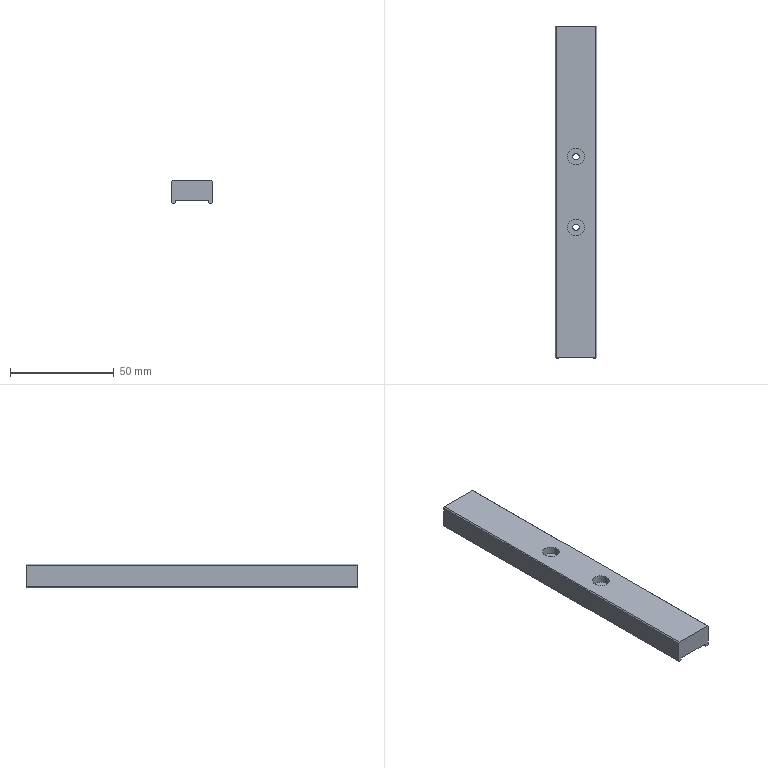Part | NX | features EXTRUDE 3, DATUM_CSYS 1 | 1 solid | 22 faces | box 20.2 x 160 x 11.5 mm | volume 32690 mm3 | plane 18 | cylinder 4 | commonest cylinder face diameters 3 x2 8 x2
STEP:
#1=CARTESIAN_POINT('',(4558.975,6805.349,0.));
#2=VERTEX_POINT('',#1);
#3=CARTESIAN_POINT('',(4578.175,6805.349,0.));
#4=VERTEX_POINT('',#3);
#5=CARTESIAN_POINT('',(4558.975,6805.349,0.));
#6=DIRECTION('',(1.,0.,0.));
#7=VECTOR('',#6,1000.);
#8=LINE('',#5,#7);
#9=EDGE_CURVE('',#2,#4,#8,.T.);
#10=ORIENTED_EDGE('',*,*,#9,.T.);
#11=CARTESIAN_POINT('',(4578.175,6965.349,0.));
#12=VERTEX_POINT('',#11);
#13=CARTESIAN_POINT('',(4578.175,6965.349,0.));
#14=DIRECTION('',(0.,-1.,0.));
#15=VECTOR('',#14,1000.);
#16=LINE('',#13,#15);
#17=EDGE_CURVE('',#12,#4,#16,.T.);
#18=ORIENTED_EDGE('',*,*,#17,.F.);
#19=CARTESIAN_POINT('',(4558.975,6965.349,0.));
#20=VERTEX_POINT('',#19);
#21=CARTESIAN_POINT('',(4558.975,6965.349,0.));
#22=DIRECTION('',(1.,0.,0.));
#23=VECTOR('',#22,1000.);
#24=LINE('',#21,#23);
#25=EDGE_CURVE('',#20,#12,#24,.T.);
#26=ORIENTED_EDGE('',*,*,#25,.F.);
#27=CARTESIAN_POINT('',(4558.975,6965.349,0.));
#28=DIRECTION('',(0.,-1.,0.));
#29=VECTOR('',#28,1000.);
#30=LINE('',#27,#29);
#31=EDGE_CURVE('',#20,#2,#30,.T.);
#32=ORIENTED_EDGE('',*,*,#31,.T.);
#33=EDGE_LOOP('',(#10,#18,#26,#32));
#34=FACE_BOUND('',#33,.T.);
#35=CARTESIAN_POINT('',(4572.575,6902.351,0.));
#36=VERTEX_POINT('',#35);
#37=CARTESIAN_POINT('',(4568.575,6902.351,0.));
#38=DIRECTION('',(0.,0.,-1.));
#39=DIRECTION('',(1.,0.,0.));
#40=AXIS2_PLACEMENT_3D('',#37,#38,#39);
#41=CIRCLE('',#40,4.);
#42=EDGE_CURVE('',#36,#36,#41,.T.);
#43=ORIENTED_EDGE('',*,*,#42,.T.);
#44=EDGE_LOOP('',(#43));
#45=FACE_BOUND('',#44,.T.);
#46=CARTESIAN_POINT('',(4572.575,6868.351,0.));
#47=VERTEX_POINT('',#46);
#48=CARTESIAN_POINT('',(4568.575,6868.351,0.));
#49=DIRECTION('',(0.,0.,1.));
#50=DIRECTION('',(1.,0.,0.));
#51=AXIS2_PLACEMENT_3D('',#48,#49,#50);
#52=CIRCLE('',#51,4.);
#53=EDGE_CURVE('',#47,#47,#52,.T.);
#54=ORIENTED_EDGE('',*,*,#53,.F.);
#55=EDGE_LOOP('',(#54));
#56=FACE_BOUND('',#55,.T.);
#57=CARTESIAN_POINT('',(4558.975,6965.349,0.));
#58=DIRECTION('',(0.,0.,-1.));
#59=DIRECTION('',(-1.,0.,0.));
#60=AXIS2_PLACEMENT_3D('',#57,#58,#59);
#61=PLANE('',#60);
#62=ADVANCED_FACE('',(#34,#45,#56),#61,.F.);
#63=CARTESIAN_POINT('',(4570.075,6868.351,-10.));
#64=VERTEX_POINT('',#63);
#65=CARTESIAN_POINT('',(4568.575,6868.351,-10.));
#66=DIRECTION('',(0.,0.,1.));
#67=DIRECTION('',(1.,0.,0.));
#68=AXIS2_PLACEMENT_3D('',#65,#66,#67);
#69=CIRCLE('',#68,1.5);
#70=EDGE_CURVE('',#64,#64,#69,.F.);
#71=ORIENTED_EDGE('',*,*,#70,.T.);
#72=EDGE_LOOP('',(#71));
#73=FACE_BOUND('',#72,.T.);
#74=CARTESIAN_POINT('',(4570.075,6868.351,-3.8));
#75=VERTEX_POINT('',#74);
#76=CARTESIAN_POINT('',(4568.575,6868.351,-3.8));
#77=DIRECTION('',(0.,0.,1.));
#78=DIRECTION('',(1.,0.,0.));
#79=AXIS2_PLACEMENT_3D('',#76,#77,#78);
#80=CIRCLE('',#79,1.5);
#81=EDGE_CURVE('',#75,#75,#80,.F.);
#82=ORIENTED_EDGE('',*,*,#81,.F.);
#83=EDGE_LOOP('',(#82));
#84=FACE_BOUND('',#83,.T.);
#85=CARTESIAN_POINT('',(4568.575,6868.351,-55000.));
#86=DIRECTION('',(0.,0.,1.));
#87=DIRECTION('',(1.,0.,0.));
#88=AXIS2_PLACEMENT_3D('',#85,#86,#87);
#89=CYLINDRICAL_SURFACE('',#88,1.5);
#90=ADVANCED_FACE('',(#73,#84),#89,.F.);
#91=CARTESIAN_POINT('',(4570.075,6902.351,-10.));
#92=VERTEX_POINT('',#91);
#93=CARTESIAN_POINT('',(4568.575,6902.351,-10.));
#94=DIRECTION('',(0.,0.,1.));
#95=DIRECTION('',(1.,0.,0.));
#96=AXIS2_PLACEMENT_3D('',#93,#94,#95);
#97=CIRCLE('',#96,1.5);
#98=EDGE_CURVE('',#92,#92,#97,.T.);
#99=ORIENTED_EDGE('',*,*,#98,.T.);
#100=EDGE_LOOP('',(#99));
#101=FACE_BOUND('',#100,.T.);
#102=CARTESIAN_POINT('',(4576.675,6805.349,-10.));
#103=VERTEX_POINT('',#102);
#104=CARTESIAN_POINT('',(4560.475,6805.349,-10.));
#105=VERTEX_POINT('',#104);
#106=CARTESIAN_POINT('',(4576.675,6805.349,-10.));
#107=DIRECTION('',(-1.,0.,0.));
#108=VECTOR('',#107,1000.);
#109=LINE('',#106,#108);
#110=EDGE_CURVE('',#103,#105,#109,.T.);
#111=ORIENTED_EDGE('',*,*,#110,.T.);
#112=CARTESIAN_POINT('',(4560.475,6965.349,-10.));
#113=VERTEX_POINT('',#112);
#114=CARTESIAN_POINT('',(4560.475,6965.349,-10.));
#115=DIRECTION('',(0.,-1.,0.));
#116=VECTOR('',#115,1000.);
#117=LINE('',#114,#116);
#118=EDGE_CURVE('',#113,#105,#117,.T.);
#119=ORIENTED_EDGE('',*,*,#118,.F.);
#120=CARTESIAN_POINT('',(4576.675,6965.349,-10.));
#121=VERTEX_POINT('',#120);
#122=CARTESIAN_POINT('',(4576.675,6965.349,-10.));
#123=DIRECTION('',(-1.,0.,0.));
#124=VECTOR('',#123,1000.);
#125=LINE('',#122,#124);
#126=EDGE_CURVE('',#121,#113,#125,.T.);
#127=ORIENTED_EDGE('',*,*,#126,.F.);
#128=CARTESIAN_POINT('',(4576.675,6965.349,-10.));
#129=DIRECTION('',(0.,-1.,0.));
#130=VECTOR('',#129,1000.);
#131=LINE('',#128,#130);
#132=EDGE_CURVE('',#121,#103,#131,.T.);
#133=ORIENTED_EDGE('',*,*,#132,.T.);
#134=EDGE_LOOP('',(#111,#119,#127,#133));
#135=FACE_BOUND('',#134,.T.);
#136=ORIENTED_EDGE('',*,*,#70,.F.);
#137=EDGE_LOOP('',(#136));
#138=FACE_BOUND('',#137,.T.);
#139=CARTESIAN_POINT('',(4576.675,6965.349,-10.));
#140=DIRECTION('',(0.,0.,1.));
#141=DIRECTION('',(1.,0.,0.));
#142=AXIS2_PLACEMENT_3D('',#139,#140,#141);
#143=PLANE('',#142);
#144=ADVANCED_FACE('',(#101,#135,#138),#143,.F.);
#145=CARTESIAN_POINT('',(4578.675,6805.349,-0.5));
#146=VERTEX_POINT('',#145);
#147=CARTESIAN_POINT('',(4578.175,6805.349,0.));
#148=DIRECTION('',(0.7071,0.,-0.7071));
#149=VECTOR('',#148,1000.);
#150=LINE('',#147,#149);
#151=EDGE_CURVE('',#4,#146,#150,.T.);
#152=ORIENTED_EDGE('',*,*,#151,.T.);
#153=CARTESIAN_POINT('',(4578.675,6965.349,-0.5));
#154=VERTEX_POINT('',#153);
#155=CARTESIAN_POINT('',(4578.675,6965.349,-0.5));
#156=DIRECTION('',(0.,-1.,0.));
#157=VECTOR('',#156,1000.);
#158=LINE('',#155,#157);
#159=EDGE_CURVE('',#154,#146,#158,.T.);
#160=ORIENTED_EDGE('',*,*,#159,.F.);
#161=CARTESIAN_POINT('',(4578.175,6965.349,0.));
#162=DIRECTION('',(0.7071,0.,-0.7071));
#163=VECTOR('',#162,1000.);
#164=LINE('',#161,#163);
#165=EDGE_CURVE('',#12,#154,#164,.T.);
#166=ORIENTED_EDGE('',*,*,#165,.F.);
#167=ORIENTED_EDGE('',*,*,#17,.T.);
#168=EDGE_LOOP('',(#152,#160,#166,#167));
#169=FACE_BOUND('',#168,.T.);
#170=CARTESIAN_POINT('',(4578.175,6965.349,0.));
#171=DIRECTION('',(-0.7071,0.,-0.7071));
#172=DIRECTION('',(-0.7071,0.,0.7071));
#173=AXIS2_PLACEMENT_3D('',#170,#171,#172);
#174=PLANE('',#173);
#175=ADVANCED_FACE('',(#169),#174,.F.);
#176=CARTESIAN_POINT('',(4578.675,6805.349,-11.));
#177=VERTEX_POINT('',#176);
#178=CARTESIAN_POINT('',(4578.675,6805.349,-0.5));
#179=DIRECTION('',(0.,0.,-1.));
#180=VECTOR('',#179,1000.);
#181=LINE('',#178,#180);
#182=EDGE_CURVE('',#146,#177,#181,.T.);
#183=ORIENTED_EDGE('',*,*,#182,.T.);
#184=CARTESIAN_POINT('',(4578.675,6965.349,-11.));
#185=VERTEX_POINT('',#184);
#186=CARTESIAN_POINT('',(4578.675,6965.349,-11.));
#187=DIRECTION('',(0.,-1.,0.));
#188=VECTOR('',#187,1000.);
#189=LINE('',#186,#188);
#190=EDGE_CURVE('',#185,#177,#189,.T.);
#191=ORIENTED_EDGE('',*,*,#190,.F.);
#192=CARTESIAN_POINT('',(4578.675,6965.349,-0.5));
#193=DIRECTION('',(0.,0.,-1.));
#194=VECTOR('',#193,1000.);
#195=LINE('',#192,#194);
#196=EDGE_CURVE('',#154,#185,#195,.T.);
#197=ORIENTED_EDGE('',*,*,#196,.F.);
#198=ORIENTED_EDGE('',*,*,#159,.T.);
#199=EDGE_LOOP('',(#183,#191,#197,#198));
#200=FACE_BOUND('',#199,.T.);
#201=CARTESIAN_POINT('',(4578.675,6965.349,-0.5));
#202=DIRECTION('',(-1.,0.,0.));
#203=DIRECTION('',(0.,0.,1.));
#204=AXIS2_PLACEMENT_3D('',#201,#202,#203);
#205=PLANE('',#204);
#206=ADVANCED_FACE('',(#200),#205,.F.);
#207=CARTESIAN_POINT('',(4578.175,6805.349,-11.5));
#208=VERTEX_POINT('',#207);
#209=CARTESIAN_POINT('',(4578.675,6805.349,-11.));
#210=DIRECTION('',(-0.7071,0.,-0.7071));
#211=VECTOR('',#210,1000.);
#212=LINE('',#209,#211);
#213=EDGE_CURVE('',#177,#208,#212,.T.);
#214=ORIENTED_EDGE('',*,*,#213,.T.);
#215=CARTESIAN_POINT('',(4578.175,6965.349,-11.5));
#216=VERTEX_POINT('',#215);
#217=CARTESIAN_POINT('',(4578.175,6965.349,-11.5));
#218=DIRECTION('',(0.,-1.,0.));
#219=VECTOR('',#218,1000.);
#220=LINE('',#217,#219);
#221=EDGE_CURVE('',#216,#208,#220,.T.);
#222=ORIENTED_EDGE('',*,*,#221,.F.);
#223=CARTESIAN_POINT('',(4578.675,6965.349,-11.));
#224=DIRECTION('',(-0.7071,0.,-0.7071));
#225=VECTOR('',#224,1000.);
#226=LINE('',#223,#225);
#227=EDGE_CURVE('',#185,#216,#226,.T.);
#228=ORIENTED_EDGE('',*,*,#227,.F.);
#229=ORIENTED_EDGE('',*,*,#190,.T.);
#230=EDGE_LOOP('',(#214,#222,#228,#229));
#231=FACE_BOUND('',#230,.T.);
#232=CARTESIAN_POINT('',(4578.675,6965.349,-11.));
#233=DIRECTION('',(-0.7071,0.,0.7071));
#234=DIRECTION('',(0.7071,0.,0.7071));
#235=AXIS2_PLACEMENT_3D('',#232,#233,#234);
#236=PLANE('',#235);
#237=ADVANCED_FACE('',(#231),#236,.F.);
#238=CARTESIAN_POINT('',(4577.175,6805.349,-11.5));
#239=VERTEX_POINT('',#238);
#240=CARTESIAN_POINT('',(4578.175,6805.349,-11.5));
#241=DIRECTION('',(-1.,0.,0.));
#242=VECTOR('',#241,1000.);
#243=LINE('',#240,#242);
#244=EDGE_CURVE('',#208,#239,#243,.T.);
#245=ORIENTED_EDGE('',*,*,#244,.T.);
#246=CARTESIAN_POINT('',(4577.175,6965.349,-11.5));
#247=VERTEX_POINT('',#246);
#248=CARTESIAN_POINT('',(4577.175,6965.349,-11.5));
#249=DIRECTION('',(0.,-1.,0.));
#250=VECTOR('',#249,1000.);
#251=LINE('',#248,#250);
#252=EDGE_CURVE('',#247,#239,#251,.T.);
#253=ORIENTED_EDGE('',*,*,#252,.F.);
#254=CARTESIAN_POINT('',(4578.175,6965.349,-11.5));
#255=DIRECTION('',(-1.,0.,0.));
#256=VECTOR('',#255,1000.);
#257=LINE('',#254,#256);
#258=EDGE_CURVE('',#216,#247,#257,.T.);
#259=ORIENTED_EDGE('',*,*,#258,.F.);
#260=ORIENTED_EDGE('',*,*,#221,.T.);
#261=EDGE_LOOP('',(#245,#253,#259,#260));
#262=FACE_BOUND('',#261,.T.);
#263=CARTESIAN_POINT('',(4578.175,6965.349,-11.5));
#264=DIRECTION('',(0.,0.,1.));
#265=DIRECTION('',(1.,0.,0.));
#266=AXIS2_PLACEMENT_3D('',#263,#264,#265);
#267=PLANE('',#266);
#268=ADVANCED_FACE('',(#262),#267,.F.);
#269=CARTESIAN_POINT('',(4576.675,6805.349,-11.));
#270=VERTEX_POINT('',#269);
#271=CARTESIAN_POINT('',(4577.175,6805.349,-11.5));
#272=DIRECTION('',(-0.7071,0.,0.7071));
#273=VECTOR('',#272,1000.);
#274=LINE('',#271,#273);
#275=EDGE_CURVE('',#239,#270,#274,.T.);
#276=ORIENTED_EDGE('',*,*,#275,.T.);
#277=CARTESIAN_POINT('',(4576.675,6965.349,-11.));
#278=VERTEX_POINT('',#277);
#279=CARTESIAN_POINT('',(4576.675,6965.349,-11.));
#280=DIRECTION('',(0.,-1.,0.));
#281=VECTOR('',#280,1000.);
#282=LINE('',#279,#281);
#283=EDGE_CURVE('',#278,#270,#282,.T.);
#284=ORIENTED_EDGE('',*,*,#283,.F.);
#285=CARTESIAN_POINT('',(4577.175,6965.349,-11.5));
#286=DIRECTION('',(-0.7071,0.,0.7071));
#287=VECTOR('',#286,1000.);
#288=LINE('',#285,#287);
#289=EDGE_CURVE('',#247,#278,#288,.T.);
#290=ORIENTED_EDGE('',*,*,#289,.F.);
#291=ORIENTED_EDGE('',*,*,#252,.T.);
#292=EDGE_LOOP('',(#276,#284,#290,#291));
#293=FACE_BOUND('',#292,.T.);
#294=CARTESIAN_POINT('',(4577.175,6965.349,-11.5));
#295=DIRECTION('',(0.7071,0.,0.7071));
#296=DIRECTION('',(0.7071,0.,-0.7071));
#297=AXIS2_PLACEMENT_3D('',#294,#295,#296);
#298=PLANE('',#297);
#299=ADVANCED_FACE('',(#293),#298,.F.);
#300=CARTESIAN_POINT('',(4576.675,6805.349,-11.));
#301=DIRECTION('',(0.,0.,1.));
#302=VECTOR('',#301,1000.);
#303=LINE('',#300,#302);
#304=EDGE_CURVE('',#270,#103,#303,.T.);
#305=ORIENTED_EDGE('',*,*,#304,.T.);
#306=ORIENTED_EDGE('',*,*,#132,.F.);
#307=CARTESIAN_POINT('',(4576.675,6965.349,-11.));
#308=DIRECTION('',(0.,0.,1.));
#309=VECTOR('',#308,1000.);
#310=LINE('',#307,#309);
#311=EDGE_CURVE('',#278,#121,#310,.T.);
#312=ORIENTED_EDGE('',*,*,#311,.F.);
#313=ORIENTED_EDGE('',*,*,#283,.T.);
#314=EDGE_LOOP('',(#305,#306,#312,#313));
#315=FACE_BOUND('',#314,.T.);
#316=CARTESIAN_POINT('',(4576.675,6965.349,-11.));
#317=DIRECTION('',(1.,0.,0.));
#318=DIRECTION('',(0.,0.,-1.));
#319=AXIS2_PLACEMENT_3D('',#316,#317,#318);
#320=PLANE('',#319);
#321=ADVANCED_FACE('',(#315),#320,.F.);
#322=CARTESIAN_POINT('',(4560.475,6805.349,-11.));
#323=VERTEX_POINT('',#322);
#324=CARTESIAN_POINT('',(4560.475,6805.349,-10.));
#325=DIRECTION('',(0.,0.,-1.));
#326=VECTOR('',#325,1000.);
#327=LINE('',#324,#326);
#328=EDGE_CURVE('',#105,#323,#327,.T.);
#329=ORIENTED_EDGE('',*,*,#328,.T.);
#330=CARTESIAN_POINT('',(4560.475,6965.349,-11.));
#331=VERTEX_POINT('',#330);
#332=CARTESIAN_POINT('',(4560.475,6965.349,-11.));
#333=DIRECTION('',(0.,-1.,0.));
#334=VECTOR('',#333,1000.);
#335=LINE('',#332,#334);
#336=EDGE_CURVE('',#331,#323,#335,.T.);
#337=ORIENTED_EDGE('',*,*,#336,.F.);
#338=CARTESIAN_POINT('',(4560.475,6965.349,-10.));
#339=DIRECTION('',(0.,0.,-1.));
#340=VECTOR('',#339,1000.);
#341=LINE('',#338,#340);
#342=EDGE_CURVE('',#113,#331,#341,.T.);
#343=ORIENTED_EDGE('',*,*,#342,.F.);
#344=ORIENTED_EDGE('',*,*,#118,.T.);
#345=EDGE_LOOP('',(#329,#337,#343,#344));
#346=FACE_BOUND('',#345,.T.);
#347=CARTESIAN_POINT('',(4560.475,6965.349,-10.));
#348=DIRECTION('',(-1.,0.,0.));
#349=DIRECTION('',(0.,0.,1.));
#350=AXIS2_PLACEMENT_3D('',#347,#348,#349);
#351=PLANE('',#350);
#352=ADVANCED_FACE('',(#346),#351,.F.);
#353=CARTESIAN_POINT('',(4559.975,6805.349,-11.5));
#354=VERTEX_POINT('',#353);
#355=CARTESIAN_POINT('',(4560.475,6805.349,-11.));
#356=DIRECTION('',(-0.7071,0.,-0.7071));
#357=VECTOR('',#356,1000.);
#358=LINE('',#355,#357);
#359=EDGE_CURVE('',#323,#354,#358,.T.);
#360=ORIENTED_EDGE('',*,*,#359,.T.);
#361=CARTESIAN_POINT('',(4559.975,6965.349,-11.5));
#362=VERTEX_POINT('',#361);
#363=CARTESIAN_POINT('',(4559.975,6965.349,-11.5));
#364=DIRECTION('',(0.,-1.,0.));
#365=VECTOR('',#364,1000.);
#366=LINE('',#363,#365);
#367=EDGE_CURVE('',#362,#354,#366,.T.);
#368=ORIENTED_EDGE('',*,*,#367,.F.);
#369=CARTESIAN_POINT('',(4560.475,6965.349,-11.));
#370=DIRECTION('',(-0.7071,0.,-0.7071));
#371=VECTOR('',#370,1000.);
#372=LINE('',#369,#371);
#373=EDGE_CURVE('',#331,#362,#372,.T.);
#374=ORIENTED_EDGE('',*,*,#373,.F.);
#375=ORIENTED_EDGE('',*,*,#336,.T.);
#376=EDGE_LOOP('',(#360,#368,#374,#375));
#377=FACE_BOUND('',#376,.T.);
#378=CARTESIAN_POINT('',(4560.475,6965.349,-11.));
#379=DIRECTION('',(-0.7071,0.,0.7071));
#380=DIRECTION('',(0.7071,0.,0.7071));
#381=AXIS2_PLACEMENT_3D('',#378,#379,#380);
#382=PLANE('',#381);
#383=ADVANCED_FACE('',(#377),#382,.F.);
#384=CARTESIAN_POINT('',(4558.975,6805.349,-11.5));
#385=VERTEX_POINT('',#384);
#386=CARTESIAN_POINT('',(4559.975,6805.349,-11.5));
#387=DIRECTION('',(-1.,0.,0.));
#388=VECTOR('',#387,1000.);
#389=LINE('',#386,#388);
#390=EDGE_CURVE('',#354,#385,#389,.T.);
#391=ORIENTED_EDGE('',*,*,#390,.T.);
#392=CARTESIAN_POINT('',(4558.975,6965.349,-11.5));
#393=VERTEX_POINT('',#392);
#394=CARTESIAN_POINT('',(4558.975,6965.349,-11.5));
#395=DIRECTION('',(0.,-1.,0.));
#396=VECTOR('',#395,1000.);
#397=LINE('',#394,#396);
#398=EDGE_CURVE('',#393,#385,#397,.T.);
#399=ORIENTED_EDGE('',*,*,#398,.F.);
#400=CARTESIAN_POINT('',(4559.975,6965.349,-11.5));
#401=DIRECTION('',(-1.,0.,0.));
#402=VECTOR('',#401,1000.);
#403=LINE('',#400,#402);
#404=EDGE_CURVE('',#362,#393,#403,.T.);
#405=ORIENTED_EDGE('',*,*,#404,.F.);
#406=ORIENTED_EDGE('',*,*,#367,.T.);
#407=EDGE_LOOP('',(#391,#399,#405,#406));
#408=FACE_BOUND('',#407,.T.);
#409=CARTESIAN_POINT('',(4559.975,6965.349,-11.5));
#410=DIRECTION('',(0.,0.,1.));
#411=DIRECTION('',(1.,0.,0.));
#412=AXIS2_PLACEMENT_3D('',#409,#410,#411);
#413=PLANE('',#412);
#414=ADVANCED_FACE('',(#408),#413,.F.);
#415=CARTESIAN_POINT('',(4558.475,6805.349,-11.));
#416=VERTEX_POINT('',#415);
#417=CARTESIAN_POINT('',(4558.975,6805.349,-11.5));
#418=DIRECTION('',(-0.7071,0.,0.7071));
#419=VECTOR('',#418,1000.);
#420=LINE('',#417,#419);
#421=EDGE_CURVE('',#385,#416,#420,.T.);
#422=ORIENTED_EDGE('',*,*,#421,.T.);
#423=CARTESIAN_POINT('',(4558.475,6965.349,-11.));
#424=VERTEX_POINT('',#423);
#425=CARTESIAN_POINT('',(4558.475,6965.349,-11.));
#426=DIRECTION('',(0.,-1.,0.));
#427=VECTOR('',#426,1000.);
#428=LINE('',#425,#427);
#429=EDGE_CURVE('',#424,#416,#428,.T.);
#430=ORIENTED_EDGE('',*,*,#429,.F.);
#431=CARTESIAN_POINT('',(4558.975,6965.349,-11.5));
#432=DIRECTION('',(-0.7071,0.,0.7071));
#433=VECTOR('',#432,1000.);
#434=LINE('',#431,#433);
#435=EDGE_CURVE('',#393,#424,#434,.T.);
#436=ORIENTED_EDGE('',*,*,#435,.F.);
#437=ORIENTED_EDGE('',*,*,#398,.T.);
#438=EDGE_LOOP('',(#422,#430,#436,#437));
#439=FACE_BOUND('',#438,.T.);
#440=CARTESIAN_POINT('',(4558.975,6965.349,-11.5));
#441=DIRECTION('',(0.7071,0.,0.7071));
#442=DIRECTION('',(0.7071,0.,-0.7071));
#443=AXIS2_PLACEMENT_3D('',#440,#441,#442);
#444=PLANE('',#443);
#445=ADVANCED_FACE('',(#439),#444,.F.);
#446=CARTESIAN_POINT('',(4558.475,6805.349,-0.5));
#447=VERTEX_POINT('',#446);
#448=CARTESIAN_POINT('',(4558.475,6805.349,-11.));
#449=DIRECTION('',(0.,0.,1.));
#450=VECTOR('',#449,1000.);
#451=LINE('',#448,#450);
#452=EDGE_CURVE('',#416,#447,#451,.T.);
#453=ORIENTED_EDGE('',*,*,#452,.T.);
#454=CARTESIAN_POINT('',(4558.475,6965.349,-0.5));
#455=VERTEX_POINT('',#454);
#456=CARTESIAN_POINT('',(4558.475,6965.349,-0.5));
#457=DIRECTION('',(0.,-1.,0.));
#458=VECTOR('',#457,1000.);
#459=LINE('',#456,#458);
#460=EDGE_CURVE('',#455,#447,#459,.T.);
#461=ORIENTED_EDGE('',*,*,#460,.F.);
#462=CARTESIAN_POINT('',(4558.475,6965.349,-11.));
#463=DIRECTION('',(0.,0.,1.));
#464=VECTOR('',#463,1000.);
#465=LINE('',#462,#464);
#466=EDGE_CURVE('',#424,#455,#465,.T.);
#467=ORIENTED_EDGE('',*,*,#466,.F.);
#468=ORIENTED_EDGE('',*,*,#429,.T.);
#469=EDGE_LOOP('',(#453,#461,#467,#468));
#470=FACE_BOUND('',#469,.T.);
#471=CARTESIAN_POINT('',(4558.475,6965.349,-11.));
#472=DIRECTION('',(1.,0.,0.));
#473=DIRECTION('',(0.,0.,-1.));
#474=AXIS2_PLACEMENT_3D('',#471,#472,#473);
#475=PLANE('',#474);
#476=ADVANCED_FACE('',(#470),#475,.F.);
#477=CARTESIAN_POINT('',(4558.475,6805.349,-0.5));
#478=DIRECTION('',(0.7071,0.,0.7071));
#479=VECTOR('',#478,1000.);
#480=LINE('',#477,#479);
#481=EDGE_CURVE('',#447,#2,#480,.T.);
#482=ORIENTED_EDGE('',*,*,#481,.T.);
#483=ORIENTED_EDGE('',*,*,#31,.F.);
#484=CARTESIAN_POINT('',(4558.475,6965.349,-0.5));
#485=DIRECTION('',(0.7071,0.,0.7071));
#486=VECTOR('',#485,1000.);
#487=LINE('',#484,#486);
#488=EDGE_CURVE('',#455,#20,#487,.T.);
#489=ORIENTED_EDGE('',*,*,#488,.F.);
#490=ORIENTED_EDGE('',*,*,#460,.T.);
#491=EDGE_LOOP('',(#482,#483,#489,#490));
#492=FACE_BOUND('',#491,.T.);
#493=CARTESIAN_POINT('',(4558.475,6965.349,-0.5));
#494=DIRECTION('',(0.7071,0.,-0.7071));
#495=DIRECTION('',(-0.7071,0.,-0.7071));
#496=AXIS2_PLACEMENT_3D('',#493,#494,#495);
#497=PLANE('',#496);
#498=ADVANCED_FACE('',(#492),#497,.F.);
#499=ORIENTED_EDGE('',*,*,#165,.T.);
#500=ORIENTED_EDGE('',*,*,#196,.T.);
#501=ORIENTED_EDGE('',*,*,#227,.T.);
#502=ORIENTED_EDGE('',*,*,#258,.T.);
#503=ORIENTED_EDGE('',*,*,#289,.T.);
#504=ORIENTED_EDGE('',*,*,#311,.T.);
#505=ORIENTED_EDGE('',*,*,#126,.T.);
#506=ORIENTED_EDGE('',*,*,#342,.T.);
#507=ORIENTED_EDGE('',*,*,#373,.T.);
#508=ORIENTED_EDGE('',*,*,#404,.T.);
#509=ORIENTED_EDGE('',*,*,#435,.T.);
#510=ORIENTED_EDGE('',*,*,#466,.T.);
#511=ORIENTED_EDGE('',*,*,#488,.T.);
#512=ORIENTED_EDGE('',*,*,#25,.T.);
#513=EDGE_LOOP('',(#499,#500,#501,#502,#503,#504,#505,#506,#507,#508,#509,#510,#511,#512));
#514=FACE_BOUND('',#513,.T.);
#515=CARTESIAN_POINT('',(0.,6965.349,0.));
#516=DIRECTION('',(0.,1.,0.));
#517=DIRECTION('',(0.,0.,1.));
#518=AXIS2_PLACEMENT_3D('',#515,#516,#517);
#519=PLANE('',#518);
#520=ADVANCED_FACE('',(#514),#519,.T.);
#521=ORIENTED_EDGE('',*,*,#151,.F.);
#522=ORIENTED_EDGE('',*,*,#9,.F.);
#523=ORIENTED_EDGE('',*,*,#481,.F.);
#524=ORIENTED_EDGE('',*,*,#452,.F.);
#525=ORIENTED_EDGE('',*,*,#421,.F.);
#526=ORIENTED_EDGE('',*,*,#390,.F.);
#527=ORIENTED_EDGE('',*,*,#359,.F.);
#528=ORIENTED_EDGE('',*,*,#328,.F.);
#529=ORIENTED_EDGE('',*,*,#110,.F.);
#530=ORIENTED_EDGE('',*,*,#304,.F.);
#531=ORIENTED_EDGE('',*,*,#275,.F.);
#532=ORIENTED_EDGE('',*,*,#244,.F.);
#533=ORIENTED_EDGE('',*,*,#213,.F.);
#534=ORIENTED_EDGE('',*,*,#182,.F.);
#535=EDGE_LOOP('',(#521,#522,#523,#524,#525,#526,#527,#528,#529,#530,#531,#532,#533,#534));
#536=FACE_BOUND('',#535,.T.);
#537=CARTESIAN_POINT('',(0.,6805.349,0.));
#538=DIRECTION('',(0.,1.,0.));
#539=DIRECTION('',(0.,0.,1.));
#540=AXIS2_PLACEMENT_3D('',#537,#538,#539);
#541=PLANE('',#540);
#542=ADVANCED_FACE('',(#536),#541,.F.);
#543=CARTESIAN_POINT('',(4567.075,6902.351,-3.8));
#544=VERTEX_POINT('',#543);
#545=CARTESIAN_POINT('',(4568.575,6902.351,-3.8));
#546=DIRECTION('',(0.,0.,-1.));
#547=DIRECTION('',(-1.,0.,0.));
#548=AXIS2_PLACEMENT_3D('',#545,#546,#547);
#549=CIRCLE('',#548,1.5);
#550=EDGE_CURVE('',#544,#544,#549,.T.);
#551=ORIENTED_EDGE('',*,*,#550,.F.);
#552=EDGE_LOOP('',(#551));
#553=FACE_BOUND('',#552,.T.);
#554=ORIENTED_EDGE('',*,*,#98,.F.);
#555=EDGE_LOOP('',(#554));
#556=FACE_BOUND('',#555,.T.);
#557=CARTESIAN_POINT('',(4568.575,6902.351,-55000.));
#558=DIRECTION('',(0.,0.,1.));
#559=DIRECTION('',(1.,0.,0.));
#560=AXIS2_PLACEMENT_3D('',#557,#558,#559);
#561=CYLINDRICAL_SURFACE('',#560,1.5);
#562=ADVANCED_FACE('',(#553,#556),#561,.F.);
#563=CARTESIAN_POINT('',(4572.575,6868.351,-3.8));
#564=VERTEX_POINT('',#563);
#565=CARTESIAN_POINT('',(4568.575,6868.351,-3.8));
#566=DIRECTION('',(0.,0.,1.));
#567=DIRECTION('',(1.,0.,0.));
#568=AXIS2_PLACEMENT_3D('',#565,#566,#567);
#569=CIRCLE('',#568,4.);
#570=EDGE_CURVE('',#564,#564,#569,.F.);
#571=ORIENTED_EDGE('',*,*,#570,.F.);
#572=EDGE_LOOP('',(#571));
#573=FACE_BOUND('',#572,.T.);
#574=ORIENTED_EDGE('',*,*,#81,.T.);
#575=EDGE_LOOP('',(#574));
#576=FACE_BOUND('',#575,.T.);
#577=CARTESIAN_POINT('',(4568.575,6868.351,-3.8));
#578=DIRECTION('',(0.,0.,1.));
#579=DIRECTION('',(1.,0.,0.));
#580=AXIS2_PLACEMENT_3D('',#577,#578,#579);
#581=PLANE('',#580);
#582=ADVANCED_FACE('',(#573,#576),#581,.T.);
#583=ORIENTED_EDGE('',*,*,#570,.T.);
#584=EDGE_LOOP('',(#583));
#585=FACE_BOUND('',#584,.T.);
#586=ORIENTED_EDGE('',*,*,#53,.T.);
#587=EDGE_LOOP('',(#586));
#588=FACE_BOUND('',#587,.T.);
#589=CARTESIAN_POINT('',(4568.575,6868.351,-3.8));
#590=DIRECTION('',(0.,0.,1.));
#591=DIRECTION('',(1.,0.,0.));
#592=AXIS2_PLACEMENT_3D('',#589,#590,#591);
#593=CYLINDRICAL_SURFACE('',#592,4.);
#594=ADVANCED_FACE('',(#585,#588),#593,.F.);
#595=CARTESIAN_POINT('',(4572.575,6902.351,-3.8));
#596=VERTEX_POINT('',#595);
#597=CARTESIAN_POINT('',(4568.575,6902.351,-3.8));
#598=DIRECTION('',(0.,0.,-1.));
#599=DIRECTION('',(1.,0.,0.));
#600=AXIS2_PLACEMENT_3D('',#597,#598,#599);
#601=CIRCLE('',#600,4.);
#602=EDGE_CURVE('',#596,#596,#601,.F.);
#603=ORIENTED_EDGE('',*,*,#602,.F.);
#604=EDGE_LOOP('',(#603));
#605=FACE_BOUND('',#604,.T.);
#606=ORIENTED_EDGE('',*,*,#42,.F.);
#607=EDGE_LOOP('',(#606));
#608=FACE_BOUND('',#607,.T.);
#609=CARTESIAN_POINT('',(4568.575,6902.351,-3.8));
#610=DIRECTION('',(0.,0.,1.));
#611=DIRECTION('',(1.,0.,0.));
#612=AXIS2_PLACEMENT_3D('',#609,#610,#611);
#613=CYLINDRICAL_SURFACE('',#612,4.);
#614=ADVANCED_FACE('',(#605,#608),#613,.F.);
#615=ORIENTED_EDGE('',*,*,#550,.T.);
#616=EDGE_LOOP('',(#615));
#617=FACE_BOUND('',#616,.T.);
#618=ORIENTED_EDGE('',*,*,#602,.T.);
#619=EDGE_LOOP('',(#618));
#620=FACE_BOUND('',#619,.T.);
#621=CARTESIAN_POINT('',(4568.575,6902.351,-3.8));
#622=DIRECTION('',(0.,0.,-1.));
#623=DIRECTION('',(-1.,0.,0.));
#624=AXIS2_PLACEMENT_3D('',#621,#622,#623);
#625=PLANE('',#624);
#626=ADVANCED_FACE('',(#617,#620),#625,.F.);
#627=CLOSED_SHELL('',(#62,#90,#144,#175,#206,#237,#268,#299,#321,#352,#383,#414,#445,#476,#498,#520,#542,#562,#582,#594,#614,#626));
#628=MANIFOLD_SOLID_BREP('',#627);
#629=(LENGTH_UNIT()NAMED_UNIT(*)SI_UNIT(.MILLI.,.METRE.));
#630=UNCERTAINTY_MEASURE_WITH_UNIT(LENGTH_MEASURE(0.00001),#629,'','');
#631=(NAMED_UNIT(*)PLANE_ANGLE_UNIT()SI_UNIT($,.RADIAN.));
#632=(NAMED_UNIT(*)SI_UNIT($,.STERADIAN.)SOLID_ANGLE_UNIT());
#633=(GEOMETRIC_REPRESENTATION_CONTEXT(3)GLOBAL_UNCERTAINTY_ASSIGNED_CONTEXT((#630))GLOBAL_UNIT_ASSIGNED_CONTEXT((#629,#631,#632))REPRESENTATION_CONTEXT('',''));
#634=ADVANCED_BREP_SHAPE_REPRESENTATION('',(#628),#633);